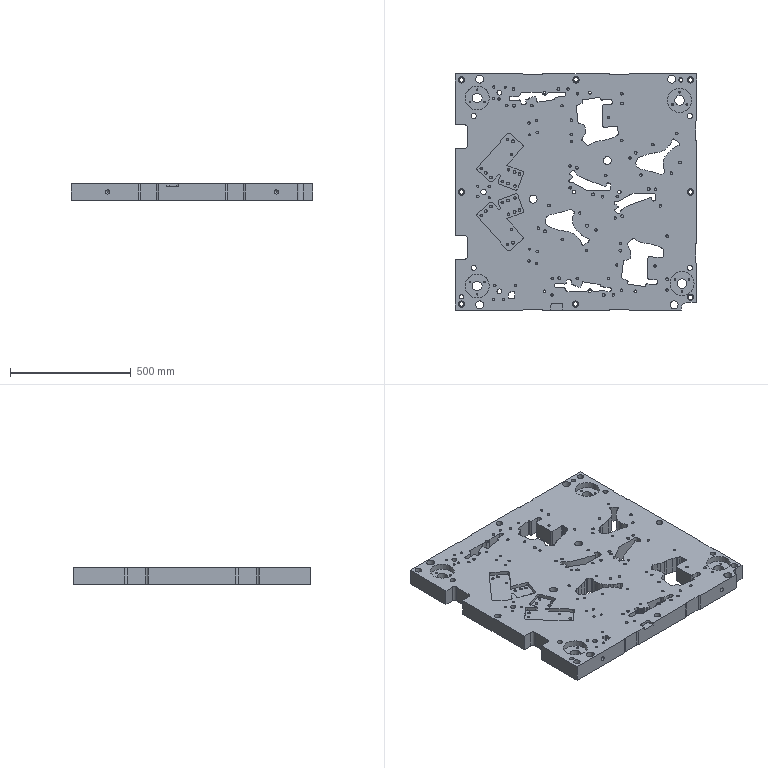Part | NX | features solid 2 | 1 solid | 654 faces | box 1000 x 980 x 69.5 mm | volume 58257679 mm3 | cylinder 360 | plane 204 | cone 83 | spline 7 | commonest cylinder face diameters 10.3 x57 8 x24 12.001 x24 16 x22 25 x16 6.8 x12